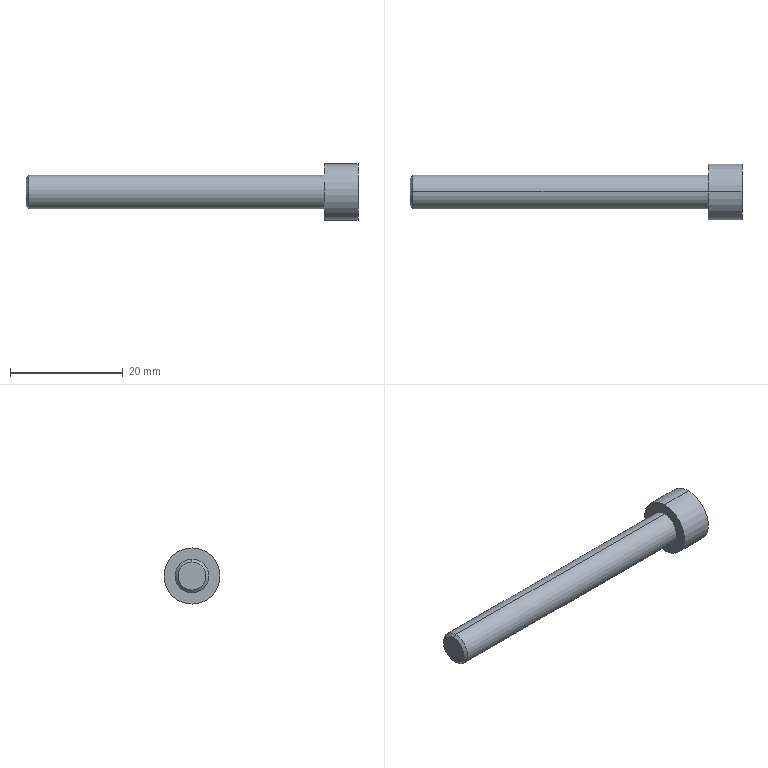Part | STEP file | 4-20.sldasm-Part-99 | 1 solid | 16 faces | box 59 x 10 x 10 mm | volume 1882 mm3 | plane 10 | cylinder 4 | cone 2 | commonest cylinder face diameters 6 x2 10 x2
STEP:
#1=CARTESIAN_POINT('',(268.,-172.617,-42.593));
#2=VERTEX_POINT('',#1);
#3=CARTESIAN_POINT('',(268.,-172.617,-52.593));
#4=VERTEX_POINT('',#3);
#5=CARTESIAN_POINT('',(268.,-172.617,-47.593));
#6=DIRECTION('',(-1.,0.,0.));
#7=DIRECTION('',(0.,0.,-1.));
#8=AXIS2_PLACEMENT_3D('',#5,#6,#7);
#9=CIRCLE('',#8,5.);
#10=EDGE_CURVE('',#2,#4,#9,.T.);
#11=ORIENTED_EDGE('',*,*,#10,.F.);
#12=CARTESIAN_POINT('',(274.,-172.617,-42.593));
#13=VERTEX_POINT('',#12);
#14=CARTESIAN_POINT('',(268.,-172.617,-42.593));
#15=DIRECTION('',(1.,0.,0.));
#16=VECTOR('',#15,1000.);
#17=LINE('',#14,#16);
#18=EDGE_CURVE('',#2,#13,#17,.T.);
#19=ORIENTED_EDGE('',*,*,#18,.T.);
#20=CARTESIAN_POINT('',(274.,-172.617,-52.593));
#21=VERTEX_POINT('',#20);
#22=CARTESIAN_POINT('',(274.,-172.617,-47.593));
#23=DIRECTION('',(-1.,0.,0.));
#24=DIRECTION('',(0.,0.,-1.));
#25=AXIS2_PLACEMENT_3D('',#22,#23,#24);
#26=CIRCLE('',#25,5.);
#27=EDGE_CURVE('',#13,#21,#26,.T.);
#28=ORIENTED_EDGE('',*,*,#27,.T.);
#29=CARTESIAN_POINT('',(268.,-172.617,-52.593));
#30=DIRECTION('',(1.,0.,0.));
#31=VECTOR('',#30,1000.);
#32=LINE('',#29,#31);
#33=EDGE_CURVE('',#4,#21,#32,.T.);
#34=ORIENTED_EDGE('',*,*,#33,.F.);
#35=EDGE_LOOP('',(#11,#19,#28,#34));
#36=FACE_OUTER_BOUND('',#35,.T.);
#37=CARTESIAN_POINT('',(268.,-172.617,-47.593));
#38=DIRECTION('',(1.,0.,0.));
#39=DIRECTION('',(0.,0.,-1.));
#40=AXIS2_PLACEMENT_3D('',#37,#38,#39);
#41=CYLINDRICAL_SURFACE('',#40,5.);
#42=ADVANCED_FACE('',(#36),#41,.T.);
#43=CARTESIAN_POINT('',(268.,-172.617,-44.593));
#44=VERTEX_POINT('',#43);
#45=CARTESIAN_POINT('',(268.,-172.617,-50.593));
#46=VERTEX_POINT('',#45);
#47=CARTESIAN_POINT('',(268.,-172.617,-47.593));
#48=DIRECTION('',(-1.,0.,0.));
#49=DIRECTION('',(0.,0.,1.));
#50=AXIS2_PLACEMENT_3D('',#47,#48,#49);
#51=CIRCLE('',#50,3.);
#52=EDGE_CURVE('',#44,#46,#51,.T.);
#53=ORIENTED_EDGE('',*,*,#52,.T.);
#54=CARTESIAN_POINT('',(215.5,-172.617,-50.593));
#55=VERTEX_POINT('',#54);
#56=CARTESIAN_POINT('',(232.,-172.617,-50.593));
#57=DIRECTION('',(-1.,0.,0.));
#58=VECTOR('',#57,1000.);
#59=LINE('',#56,#58);
#60=EDGE_CURVE('',#46,#55,#59,.T.);
#61=ORIENTED_EDGE('',*,*,#60,.T.);
#62=CARTESIAN_POINT('',(215.5,-172.617,-44.593));
#63=VERTEX_POINT('',#62);
#64=CARTESIAN_POINT('',(215.5,-172.617,-47.593));
#65=DIRECTION('',(1.,0.,0.));
#66=DIRECTION('',(0.,0.,1.));
#67=AXIS2_PLACEMENT_3D('',#64,#65,#66);
#68=CIRCLE('',#67,3.);
#69=EDGE_CURVE('',#55,#63,#68,.T.);
#70=ORIENTED_EDGE('',*,*,#69,.T.);
#71=CARTESIAN_POINT('',(232.,-172.617,-44.593));
#72=DIRECTION('',(-1.,0.,0.));
#73=VECTOR('',#72,1000.);
#74=LINE('',#71,#73);
#75=EDGE_CURVE('',#44,#63,#74,.T.);
#76=ORIENTED_EDGE('',*,*,#75,.F.);
#77=EDGE_LOOP('',(#53,#61,#70,#76));
#78=FACE_OUTER_BOUND('',#77,.T.);
#79=CARTESIAN_POINT('',(232.,-172.617,-47.593));
#80=DIRECTION('',(-1.,0.,0.));
#81=DIRECTION('',(0.,0.,1.));
#82=AXIS2_PLACEMENT_3D('',#79,#80,#81);
#83=CYLINDRICAL_SURFACE('',#82,3.);
#84=ADVANCED_FACE('',(#78),#83,.T.);
#85=CARTESIAN_POINT('',(215.,-172.617,-45.093));
#86=VERTEX_POINT('',#85);
#87=CARTESIAN_POINT('',(215.,-172.617,-50.093));
#88=VERTEX_POINT('',#87);
#89=CARTESIAN_POINT('',(215.,-172.617,-47.593));
#90=DIRECTION('',(-1.,0.,0.));
#91=DIRECTION('',(0.,-1.,0.));
#92=AXIS2_PLACEMENT_3D('',#89,#90,#91);
#93=CIRCLE('',#92,2.5);
#94=EDGE_CURVE('',#86,#88,#93,.T.);
#95=ORIENTED_EDGE('',*,*,#94,.F.);
#96=CARTESIAN_POINT('',(215.,-172.617,-45.093));
#97=DIRECTION('',(0.7071,0.,0.7071));
#98=VECTOR('',#97,1000.);
#99=LINE('',#96,#98);
#100=EDGE_CURVE('',#86,#63,#99,.T.);
#101=ORIENTED_EDGE('',*,*,#100,.T.);
#102=ORIENTED_EDGE('',*,*,#69,.F.);
#103=CARTESIAN_POINT('',(215.,-172.617,-50.093));
#104=DIRECTION('',(0.7071,0.,-0.7071));
#105=VECTOR('',#104,1000.);
#106=LINE('',#103,#105);
#107=EDGE_CURVE('',#88,#55,#106,.T.);
#108=ORIENTED_EDGE('',*,*,#107,.F.);
#109=EDGE_LOOP('',(#95,#101,#102,#108));
#110=FACE_OUTER_BOUND('',#109,.T.);
#111=CARTESIAN_POINT('',(215.,-172.617,-47.593));
#112=DIRECTION('',(1.,0.,0.));
#113=DIRECTION('',(0.,0.,-1.));
#114=AXIS2_PLACEMENT_3D('',#111,#112,#113);
#115=CONICAL_SURFACE('',#114,2.5,0.7854);
#116=ADVANCED_FACE('',(#110),#115,.T.);
#117=CARTESIAN_POINT('',(215.,-172.617,-47.593));
#118=DIRECTION('',(-1.,0.,0.));
#119=DIRECTION('',(0.,-1.,0.));
#120=AXIS2_PLACEMENT_3D('',#117,#118,#119);
#121=CIRCLE('',#120,2.5);
#122=EDGE_CURVE('',#88,#86,#121,.T.);
#123=ORIENTED_EDGE('',*,*,#122,.T.);
#124=ORIENTED_EDGE('',*,*,#94,.T.);
#125=EDGE_LOOP('',(#123,#124));
#126=FACE_OUTER_BOUND('',#125,.T.);
#127=CARTESIAN_POINT('',(215.,-106.617,-65.593));
#128=DIRECTION('',(-1.,0.,0.));
#129=DIRECTION('',(0.,-1.,0.));
#130=AXIS2_PLACEMENT_3D('',#127,#128,#129);
#131=PLANE('',#130);
#132=ADVANCED_FACE('',(#126),#131,.T.);
#133=ORIENTED_EDGE('',*,*,#100,.F.);
#134=ORIENTED_EDGE('',*,*,#122,.F.);
#135=ORIENTED_EDGE('',*,*,#107,.T.);
#136=CARTESIAN_POINT('',(215.5,-172.617,-47.593));
#137=DIRECTION('',(1.,0.,0.));
#138=DIRECTION('',(0.,0.,1.));
#139=AXIS2_PLACEMENT_3D('',#136,#137,#138);
#140=CIRCLE('',#139,3.);
#141=EDGE_CURVE('',#63,#55,#140,.T.);
#142=ORIENTED_EDGE('',*,*,#141,.F.);
#143=EDGE_LOOP('',(#133,#134,#135,#142));
#144=FACE_OUTER_BOUND('',#143,.T.);
#145=CARTESIAN_POINT('',(215.,-172.617,-47.593));
#146=DIRECTION('',(1.,0.,0.));
#147=DIRECTION('',(0.,0.,-1.));
#148=AXIS2_PLACEMENT_3D('',#145,#146,#147);
#149=CONICAL_SURFACE('',#148,2.5,0.7854);
#150=ADVANCED_FACE('',(#144),#149,.T.);
#151=ORIENTED_EDGE('',*,*,#60,.F.);
#152=CARTESIAN_POINT('',(268.,-172.617,-47.593));
#153=DIRECTION('',(-1.,0.,0.));
#154=DIRECTION('',(0.,0.,1.));
#155=AXIS2_PLACEMENT_3D('',#152,#153,#154);
#156=CIRCLE('',#155,3.);
#157=EDGE_CURVE('',#46,#44,#156,.T.);
#158=ORIENTED_EDGE('',*,*,#157,.T.);
#159=ORIENTED_EDGE('',*,*,#75,.T.);
#160=ORIENTED_EDGE('',*,*,#141,.T.);
#161=EDGE_LOOP('',(#151,#158,#159,#160));
#162=FACE_OUTER_BOUND('',#161,.T.);
#163=CARTESIAN_POINT('',(232.,-172.617,-47.593));
#164=DIRECTION('',(-1.,0.,0.));
#165=DIRECTION('',(0.,0.,1.));
#166=AXIS2_PLACEMENT_3D('',#163,#164,#165);
#167=CYLINDRICAL_SURFACE('',#166,3.);
#168=ADVANCED_FACE('',(#162),#167,.T.);
#169=CARTESIAN_POINT('',(268.,-172.617,-47.593));
#170=DIRECTION('',(-1.,0.,0.));
#171=DIRECTION('',(0.,0.,-1.));
#172=AXIS2_PLACEMENT_3D('',#169,#170,#171);
#173=CIRCLE('',#172,5.);
#174=EDGE_CURVE('',#4,#2,#173,.T.);
#175=ORIENTED_EDGE('',*,*,#174,.T.);
#176=ORIENTED_EDGE('',*,*,#10,.T.);
#177=EDGE_LOOP('',(#175,#176));
#178=FACE_OUTER_BOUND('',#177,.T.);
#179=ORIENTED_EDGE('',*,*,#52,.F.);
#180=ORIENTED_EDGE('',*,*,#157,.F.);
#181=EDGE_LOOP('',(#179,#180));
#182=FACE_BOUND('',#181,.T.);
#183=CARTESIAN_POINT('',(268.,-172.617,-47.593));
#184=DIRECTION('',(-1.,0.,0.));
#185=DIRECTION('',(0.,0.,1.));
#186=AXIS2_PLACEMENT_3D('',#183,#184,#185);
#187=PLANE('',#186);
#188=ADVANCED_FACE('',(#178,#182),#187,.T.);
#189=CARTESIAN_POINT('',(274.,-170.117,-46.15));
#190=VERTEX_POINT('',#189);
#191=CARTESIAN_POINT('',(274.,-170.117,-49.036));
#192=VERTEX_POINT('',#191);
#193=CARTESIAN_POINT('',(274.,-170.117,-46.15));
#194=DIRECTION('',(0.,0.,-1.));
#195=VECTOR('',#194,1000.);
#196=LINE('',#193,#195);
#197=EDGE_CURVE('',#190,#192,#196,.T.);
#198=ORIENTED_EDGE('',*,*,#197,.T.);
#199=CARTESIAN_POINT('',(274.,-172.617,-50.48));
#200=VERTEX_POINT('',#199);
#201=CARTESIAN_POINT('',(274.,-170.117,-49.036));
#202=DIRECTION('',(0.,-0.866,-0.5));
#203=VECTOR('',#202,1000.);
#204=LINE('',#201,#203);
#205=EDGE_CURVE('',#192,#200,#204,.T.);
#206=ORIENTED_EDGE('',*,*,#205,.T.);
#207=CARTESIAN_POINT('',(274.,-175.117,-49.036));
#208=VERTEX_POINT('',#207);
#209=CARTESIAN_POINT('',(274.,-172.617,-50.48));
#210=DIRECTION('',(0.,-0.866,0.5));
#211=VECTOR('',#210,1000.);
#212=LINE('',#209,#211);
#213=EDGE_CURVE('',#200,#208,#212,.T.);
#214=ORIENTED_EDGE('',*,*,#213,.T.);
#215=CARTESIAN_POINT('',(274.,-175.117,-46.15));
#216=VERTEX_POINT('',#215);
#217=CARTESIAN_POINT('',(274.,-175.117,-49.036));
#218=DIRECTION('',(0.,0.,1.));
#219=VECTOR('',#218,1000.);
#220=LINE('',#217,#219);
#221=EDGE_CURVE('',#208,#216,#220,.T.);
#222=ORIENTED_EDGE('',*,*,#221,.T.);
#223=CARTESIAN_POINT('',(274.,-172.617,-44.706));
#224=VERTEX_POINT('',#223);
#225=CARTESIAN_POINT('',(274.,-175.117,-46.15));
#226=DIRECTION('',(0.,0.866,0.5));
#227=VECTOR('',#226,1000.);
#228=LINE('',#225,#227);
#229=EDGE_CURVE('',#216,#224,#228,.T.);
#230=ORIENTED_EDGE('',*,*,#229,.T.);
#231=CARTESIAN_POINT('',(274.,-172.617,-44.706));
#232=DIRECTION('',(0.,0.866,-0.5));
#233=VECTOR('',#232,1000.);
#234=LINE('',#231,#233);
#235=EDGE_CURVE('',#224,#190,#234,.T.);
#236=ORIENTED_EDGE('',*,*,#235,.T.);
#237=EDGE_LOOP('',(#198,#206,#214,#222,#230,#236));
#238=FACE_BOUND('',#237,.T.);
#239=CARTESIAN_POINT('',(274.,-172.617,-47.593));
#240=DIRECTION('',(-1.,0.,0.));
#241=DIRECTION('',(0.,0.,-1.));
#242=AXIS2_PLACEMENT_3D('',#239,#240,#241);
#243=CIRCLE('',#242,5.);
#244=EDGE_CURVE('',#21,#13,#243,.T.);
#245=ORIENTED_EDGE('',*,*,#244,.F.);
#246=ORIENTED_EDGE('',*,*,#27,.F.);
#247=EDGE_LOOP('',(#245,#246));
#248=FACE_OUTER_BOUND('',#247,.T.);
#249=CARTESIAN_POINT('',(274.,-172.617,-47.593));
#250=DIRECTION('',(1.,0.,0.));
#251=DIRECTION('',(0.,0.,-1.));
#252=AXIS2_PLACEMENT_3D('',#249,#250,#251);
#253=PLANE('',#252);
#254=ADVANCED_FACE('',(#238,#248),#253,.T.);
#255=ORIENTED_EDGE('',*,*,#18,.F.);
#256=ORIENTED_EDGE('',*,*,#174,.F.);
#257=ORIENTED_EDGE('',*,*,#33,.T.);
#258=ORIENTED_EDGE('',*,*,#244,.T.);
#259=EDGE_LOOP('',(#255,#256,#257,#258));
#260=FACE_OUTER_BOUND('',#259,.T.);
#261=CARTESIAN_POINT('',(268.,-172.617,-47.593));
#262=DIRECTION('',(1.,0.,0.));
#263=DIRECTION('',(0.,0.,-1.));
#264=AXIS2_PLACEMENT_3D('',#261,#262,#263);
#265=CYLINDRICAL_SURFACE('',#264,5.);
#266=ADVANCED_FACE('',(#260),#265,.T.);
#267=ORIENTED_EDGE('',*,*,#197,.F.);
#268=CARTESIAN_POINT('',(270.04,-170.117,-46.15));
#269=VERTEX_POINT('',#268);
#270=CARTESIAN_POINT('',(270.04,-170.117,-46.15));
#271=DIRECTION('',(1.,0.,0.));
#272=VECTOR('',#271,1000.);
#273=LINE('',#270,#272);
#274=EDGE_CURVE('',#269,#190,#273,.T.);
#275=ORIENTED_EDGE('',*,*,#274,.F.);
#276=CARTESIAN_POINT('',(270.04,-170.117,-49.036));
#277=VERTEX_POINT('',#276);
#278=CARTESIAN_POINT('',(270.04,-170.117,-46.15));
#279=DIRECTION('',(0.,0.,-1.));
#280=VECTOR('',#279,1000.);
#281=LINE('',#278,#280);
#282=EDGE_CURVE('',#269,#277,#281,.T.);
#283=ORIENTED_EDGE('',*,*,#282,.T.);
#284=CARTESIAN_POINT('',(270.04,-170.117,-49.036));
#285=DIRECTION('',(1.,0.,0.));
#286=VECTOR('',#285,1000.);
#287=LINE('',#284,#286);
#288=EDGE_CURVE('',#277,#192,#287,.T.);
#289=ORIENTED_EDGE('',*,*,#288,.T.);
#290=EDGE_LOOP('',(#267,#275,#283,#289));
#291=FACE_OUTER_BOUND('',#290,.T.);
#292=CARTESIAN_POINT('',(270.04,-170.117,-46.15));
#293=DIRECTION('',(0.,1.,0.));
#294=DIRECTION('',(-1.,0.,0.));
#295=AXIS2_PLACEMENT_3D('',#292,#293,#294);
#296=PLANE('',#295);
#297=ADVANCED_FACE('',(#291),#296,.F.);
#298=ORIENTED_EDGE('',*,*,#205,.F.);
#299=ORIENTED_EDGE('',*,*,#288,.F.);
#300=CARTESIAN_POINT('',(270.04,-172.617,-50.48));
#301=VERTEX_POINT('',#300);
#302=CARTESIAN_POINT('',(270.04,-170.117,-49.036));
#303=DIRECTION('',(0.,-0.866,-0.5));
#304=VECTOR('',#303,1000.);
#305=LINE('',#302,#304);
#306=EDGE_CURVE('',#277,#301,#305,.T.);
#307=ORIENTED_EDGE('',*,*,#306,.T.);
#308=CARTESIAN_POINT('',(270.04,-172.617,-50.48));
#309=DIRECTION('',(1.,0.,0.));
#310=VECTOR('',#309,1000.);
#311=LINE('',#308,#310);
#312=EDGE_CURVE('',#301,#200,#311,.T.);
#313=ORIENTED_EDGE('',*,*,#312,.T.);
#314=EDGE_LOOP('',(#298,#299,#307,#313));
#315=FACE_OUTER_BOUND('',#314,.T.);
#316=CARTESIAN_POINT('',(270.04,-170.117,-49.036));
#317=DIRECTION('',(0.,0.5,-0.866));
#318=DIRECTION('',(0.,-0.866,-0.5));
#319=AXIS2_PLACEMENT_3D('',#316,#317,#318);
#320=PLANE('',#319);
#321=ADVANCED_FACE('',(#315),#320,.F.);
#322=ORIENTED_EDGE('',*,*,#213,.F.);
#323=ORIENTED_EDGE('',*,*,#312,.F.);
#324=CARTESIAN_POINT('',(270.04,-175.117,-49.036));
#325=VERTEX_POINT('',#324);
#326=CARTESIAN_POINT('',(270.04,-172.617,-50.48));
#327=DIRECTION('',(0.,-0.866,0.5));
#328=VECTOR('',#327,1000.);
#329=LINE('',#326,#328);
#330=EDGE_CURVE('',#301,#325,#329,.T.);
#331=ORIENTED_EDGE('',*,*,#330,.T.);
#332=CARTESIAN_POINT('',(270.04,-175.117,-49.036));
#333=DIRECTION('',(1.,0.,0.));
#334=VECTOR('',#333,1000.);
#335=LINE('',#332,#334);
#336=EDGE_CURVE('',#325,#208,#335,.T.);
#337=ORIENTED_EDGE('',*,*,#336,.T.);
#338=EDGE_LOOP('',(#322,#323,#331,#337));
#339=FACE_OUTER_BOUND('',#338,.T.);
#340=CARTESIAN_POINT('',(270.04,-172.617,-50.48));
#341=DIRECTION('',(0.,-0.5,-0.866));
#342=DIRECTION('',(0.,-0.866,0.5));
#343=AXIS2_PLACEMENT_3D('',#340,#341,#342);
#344=PLANE('',#343);
#345=ADVANCED_FACE('',(#339),#344,.F.);
#346=ORIENTED_EDGE('',*,*,#221,.F.);
#347=ORIENTED_EDGE('',*,*,#336,.F.);
#348=CARTESIAN_POINT('',(270.04,-175.117,-46.15));
#349=VERTEX_POINT('',#348);
#350=CARTESIAN_POINT('',(270.04,-175.117,-49.036));
#351=DIRECTION('',(0.,0.,1.));
#352=VECTOR('',#351,1000.);
#353=LINE('',#350,#352);
#354=EDGE_CURVE('',#325,#349,#353,.T.);
#355=ORIENTED_EDGE('',*,*,#354,.T.);
#356=CARTESIAN_POINT('',(270.04,-175.117,-46.15));
#357=DIRECTION('',(1.,0.,0.));
#358=VECTOR('',#357,1000.);
#359=LINE('',#356,#358);
#360=EDGE_CURVE('',#349,#216,#359,.T.);
#361=ORIENTED_EDGE('',*,*,#360,.T.);
#362=EDGE_LOOP('',(#346,#347,#355,#361));
#363=FACE_OUTER_BOUND('',#362,.T.);
#364=CARTESIAN_POINT('',(270.04,-175.117,-49.036));
#365=DIRECTION('',(0.,-1.,0.));
#366=DIRECTION('',(1.,0.,0.));
#367=AXIS2_PLACEMENT_3D('',#364,#365,#366);
#368=PLANE('',#367);
#369=ADVANCED_FACE('',(#363),#368,.F.);
#370=ORIENTED_EDGE('',*,*,#229,.F.);
#371=ORIENTED_EDGE('',*,*,#360,.F.);
#372=CARTESIAN_POINT('',(270.04,-172.617,-44.706));
#373=VERTEX_POINT('',#372);
#374=CARTESIAN_POINT('',(270.04,-175.117,-46.15));
#375=DIRECTION('',(0.,0.866,0.5));
#376=VECTOR('',#375,1000.);
#377=LINE('',#374,#376);
#378=EDGE_CURVE('',#349,#373,#377,.T.);
#379=ORIENTED_EDGE('',*,*,#378,.T.);
#380=CARTESIAN_POINT('',(270.04,-172.617,-44.706));
#381=DIRECTION('',(1.,0.,0.));
#382=VECTOR('',#381,1000.);
#383=LINE('',#380,#382);
#384=EDGE_CURVE('',#373,#224,#383,.T.);
#385=ORIENTED_EDGE('',*,*,#384,.T.);
#386=EDGE_LOOP('',(#370,#371,#379,#385));
#387=FACE_OUTER_BOUND('',#386,.T.);
#388=CARTESIAN_POINT('',(270.04,-175.117,-46.15));
#389=DIRECTION('',(0.,-0.5,0.866));
#390=DIRECTION('',(0.,0.866,0.5));
#391=AXIS2_PLACEMENT_3D('',#388,#389,#390);
#392=PLANE('',#391);
#393=ADVANCED_FACE('',(#387),#392,.F.);
#394=ORIENTED_EDGE('',*,*,#235,.F.);
#395=ORIENTED_EDGE('',*,*,#384,.F.);
#396=CARTESIAN_POINT('',(270.04,-172.617,-44.706));
#397=DIRECTION('',(0.,0.866,-0.5));
#398=VECTOR('',#397,1000.);
#399=LINE('',#396,#398);
#400=EDGE_CURVE('',#373,#269,#399,.T.);
#401=ORIENTED_EDGE('',*,*,#400,.T.);
#402=ORIENTED_EDGE('',*,*,#274,.T.);
#403=EDGE_LOOP('',(#394,#395,#401,#402));
#404=FACE_OUTER_BOUND('',#403,.T.);
#405=CARTESIAN_POINT('',(270.04,-172.617,-44.706));
#406=DIRECTION('',(0.,0.5,0.866));
#407=DIRECTION('',(0.,0.866,-0.5));
#408=AXIS2_PLACEMENT_3D('',#405,#406,#407);
#409=PLANE('',#408);
#410=ADVANCED_FACE('',(#404),#409,.F.);
#411=ORIENTED_EDGE('',*,*,#282,.F.);
#412=ORIENTED_EDGE('',*,*,#400,.F.);
#413=ORIENTED_EDGE('',*,*,#378,.F.);
#414=ORIENTED_EDGE('',*,*,#354,.F.);
#415=ORIENTED_EDGE('',*,*,#330,.F.);
#416=ORIENTED_EDGE('',*,*,#306,.F.);
#417=EDGE_LOOP('',(#411,#412,#413,#414,#415,#416));
#418=FACE_OUTER_BOUND('',#417,.T.);
#419=CARTESIAN_POINT('',(270.04,-170.117,-49.036));
#420=DIRECTION('',(1.,0.,0.));
#421=DIRECTION('',(0.,0.,-1.));
#422=AXIS2_PLACEMENT_3D('',#419,#420,#421);
#423=PLANE('',#422);
#424=ADVANCED_FACE('',(#418),#423,.T.);
#425=CLOSED_SHELL('',(#42,#84,#116,#132,#150,#168,#188,#254,#266,#297,#321,#345,#369,#393,#410,#424));
#426=MANIFOLD_SOLID_BREP('',#425);
#427=CARTESIAN_POINT('',(0.,0.,0.));
#428=DIRECTION('',(0.,0.,1.));
#429=DIRECTION('',(1.,0.,0.));
#430=AXIS2_PLACEMENT_3D('',#427,#428,#429);
#431=(LENGTH_UNIT()NAMED_UNIT(*)SI_UNIT(.MILLI.,.METRE.));
#432=UNCERTAINTY_MEASURE_WITH_UNIT(LENGTH_MEASURE(0.00001),#431,'','');
#433=(NAMED_UNIT(*)PLANE_ANGLE_UNIT()SI_UNIT($,.RADIAN.));
#434=(NAMED_UNIT(*)SI_UNIT($,.STERADIAN.)SOLID_ANGLE_UNIT());
#435=(GEOMETRIC_REPRESENTATION_CONTEXT(3)GLOBAL_UNCERTAINTY_ASSIGNED_CONTEXT((#432))GLOBAL_UNIT_ASSIGNED_CONTEXT((#431,#433,#434))REPRESENTATION_CONTEXT('',''));
#436=ADVANCED_BREP_SHAPE_REPRESENTATION('',(#426,#430),#435);